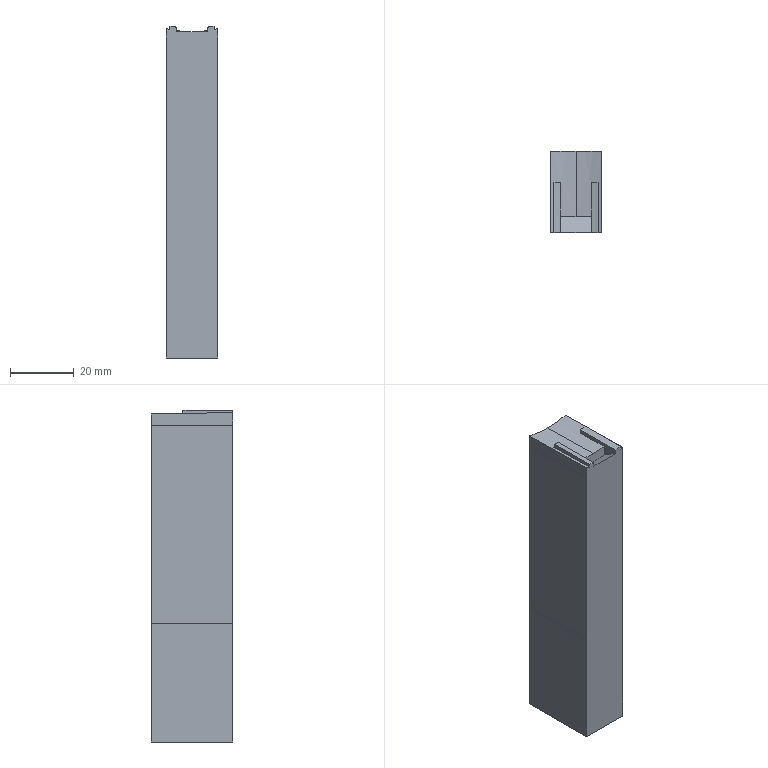Part | STEP file | Core - Tower - Drawer insert 1 - 1 cav | 1 solid | 21 faces | box 16.003 x 25.438 x 104.081 mm | volume 41692 mm3 | plane 17 | cone 2 | cylinder 2 | commonest cylinder face diameters 67.284 x2